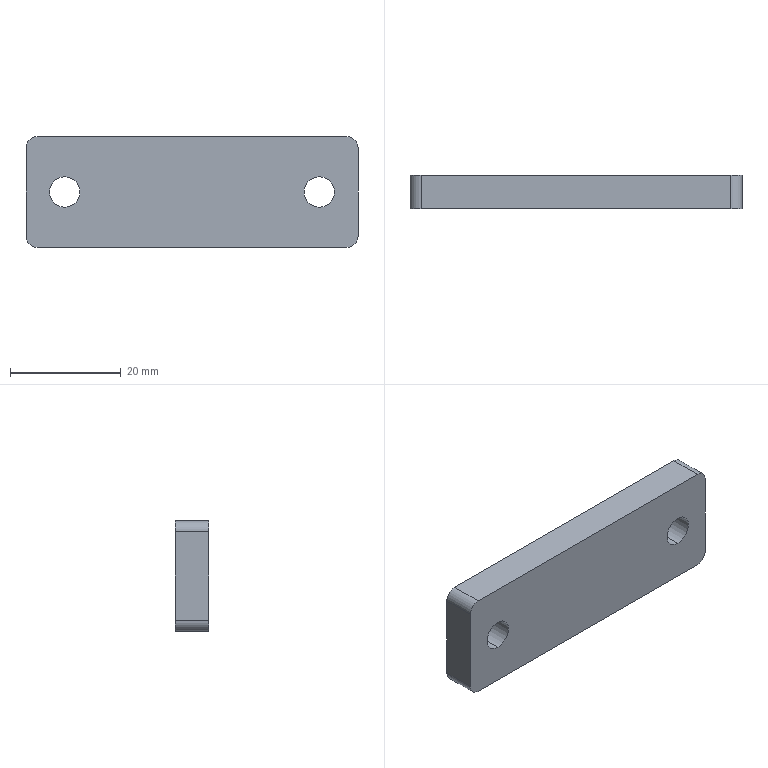Part | SolidWorks | features BaseBody 1 | 1 solid | 14 faces | box 60 x 6 x 20 mm | volume 6894 mm3 | cylinder 8 | plane 6 | commonest cylinder face diameters 4 x4 5.5 x4
STEP:
#1=CARTESIAN_POINT('',(23.,6.,2.75));
#2=VERTEX_POINT('',#1);
#3=CARTESIAN_POINT('',(23.,6.,-2.75));
#4=VERTEX_POINT('',#3);
#5=CARTESIAN_POINT('',(23.,6.,0.));
#6=DIRECTION('',(0.,-1.,0.));
#7=DIRECTION('',(0.,0.,-1.));
#8=AXIS2_PLACEMENT_3D('',#5,#6,#7);
#9=CIRCLE('',#8,2.75);
#10=EDGE_CURVE('',#2,#4,#9,.T.);
#11=ORIENTED_EDGE('',*,*,#10,.F.);
#12=CARTESIAN_POINT('',(23.,0.,2.75));
#13=VERTEX_POINT('',#12);
#14=CARTESIAN_POINT('',(23.,6.,2.75));
#15=DIRECTION('',(0.,-1.,0.));
#16=VECTOR('',#15,1000.);
#17=LINE('',#14,#16);
#18=EDGE_CURVE('',#2,#13,#17,.T.);
#19=ORIENTED_EDGE('',*,*,#18,.T.);
#20=CARTESIAN_POINT('',(23.,0.,-2.75));
#21=VERTEX_POINT('',#20);
#22=CARTESIAN_POINT('',(23.,0.,0.));
#23=DIRECTION('',(0.,1.,0.));
#24=DIRECTION('',(0.,0.,-1.));
#25=AXIS2_PLACEMENT_3D('',#22,#23,#24);
#26=CIRCLE('',#25,2.75);
#27=EDGE_CURVE('',#21,#13,#26,.T.);
#28=ORIENTED_EDGE('',*,*,#27,.F.);
#29=CARTESIAN_POINT('',(23.,6.,-2.75));
#30=DIRECTION('',(0.,-1.,0.));
#31=VECTOR('',#30,1000.);
#32=LINE('',#29,#31);
#33=EDGE_CURVE('',#4,#21,#32,.T.);
#34=ORIENTED_EDGE('',*,*,#33,.F.);
#35=EDGE_LOOP('',(#11,#19,#28,#34));
#36=FACE_OUTER_BOUND('',#35,.T.);
#37=CARTESIAN_POINT('',(23.,6.,0.));
#38=DIRECTION('',(0.,-1.,0.));
#39=DIRECTION('',(0.,0.,-1.));
#40=AXIS2_PLACEMENT_3D('',#37,#38,#39);
#41=CYLINDRICAL_SURFACE('',#40,2.75);
#42=ADVANCED_FACE('',(#36),#41,.F.);
#43=CARTESIAN_POINT('',(-23.,6.,2.75));
#44=VERTEX_POINT('',#43);
#45=CARTESIAN_POINT('',(-23.,6.,-2.75));
#46=VERTEX_POINT('',#45);
#47=CARTESIAN_POINT('',(-23.,6.,0.));
#48=DIRECTION('',(0.,-1.,0.));
#49=DIRECTION('',(0.,0.,-1.));
#50=AXIS2_PLACEMENT_3D('',#47,#48,#49);
#51=CIRCLE('',#50,2.75);
#52=EDGE_CURVE('',#44,#46,#51,.T.);
#53=ORIENTED_EDGE('',*,*,#52,.F.);
#54=CARTESIAN_POINT('',(-23.,0.,2.75));
#55=VERTEX_POINT('',#54);
#56=CARTESIAN_POINT('',(-23.,6.,2.75));
#57=DIRECTION('',(0.,-1.,0.));
#58=VECTOR('',#57,1000.);
#59=LINE('',#56,#58);
#60=EDGE_CURVE('',#44,#55,#59,.T.);
#61=ORIENTED_EDGE('',*,*,#60,.T.);
#62=CARTESIAN_POINT('',(-23.,0.,-2.75));
#63=VERTEX_POINT('',#62);
#64=CARTESIAN_POINT('',(-23.,0.,0.));
#65=DIRECTION('',(0.,1.,0.));
#66=DIRECTION('',(0.,0.,-1.));
#67=AXIS2_PLACEMENT_3D('',#64,#65,#66);
#68=CIRCLE('',#67,2.75);
#69=EDGE_CURVE('',#63,#55,#68,.T.);
#70=ORIENTED_EDGE('',*,*,#69,.F.);
#71=CARTESIAN_POINT('',(-23.,6.,-2.75));
#72=DIRECTION('',(0.,-1.,0.));
#73=VECTOR('',#72,1000.);
#74=LINE('',#71,#73);
#75=EDGE_CURVE('',#46,#63,#74,.T.);
#76=ORIENTED_EDGE('',*,*,#75,.F.);
#77=EDGE_LOOP('',(#53,#61,#70,#76));
#78=FACE_OUTER_BOUND('',#77,.T.);
#79=CARTESIAN_POINT('',(-23.,6.,0.));
#80=DIRECTION('',(0.,-1.,0.));
#81=DIRECTION('',(0.,0.,-1.));
#82=AXIS2_PLACEMENT_3D('',#79,#80,#81);
#83=CYLINDRICAL_SURFACE('',#82,2.75);
#84=ADVANCED_FACE('',(#78),#83,.F.);
#85=CARTESIAN_POINT('',(23.,6.,0.));
#86=DIRECTION('',(0.,-1.,0.));
#87=DIRECTION('',(0.,0.,-1.));
#88=AXIS2_PLACEMENT_3D('',#85,#86,#87);
#89=CIRCLE('',#88,2.75);
#90=EDGE_CURVE('',#4,#2,#89,.T.);
#91=ORIENTED_EDGE('',*,*,#90,.T.);
#92=ORIENTED_EDGE('',*,*,#10,.T.);
#93=EDGE_LOOP('',(#91,#92));
#94=FACE_BOUND('',#93,.T.);
#95=CARTESIAN_POINT('',(-30.,6.,-8.));
#96=VERTEX_POINT('',#95);
#97=CARTESIAN_POINT('',(-30.,6.,8.));
#98=VERTEX_POINT('',#97);
#99=CARTESIAN_POINT('',(-30.,6.,0.));
#100=DIRECTION('',(0.,0.,1.));
#101=VECTOR('',#100,1000.);
#102=LINE('',#99,#101);
#103=EDGE_CURVE('',#96,#98,#102,.T.);
#104=ORIENTED_EDGE('',*,*,#103,.T.);
#105=CARTESIAN_POINT('',(-28.,6.,10.));
#106=VERTEX_POINT('',#105);
#107=CARTESIAN_POINT('',(-28.,6.,8.));
#108=DIRECTION('',(0.,1.,0.));
#109=DIRECTION('',(0.,0.,-1.));
#110=AXIS2_PLACEMENT_3D('',#107,#108,#109);
#111=CIRCLE('',#110,2.);
#112=EDGE_CURVE('',#98,#106,#111,.T.);
#113=ORIENTED_EDGE('',*,*,#112,.T.);
#114=CARTESIAN_POINT('',(28.,6.,10.));
#115=VERTEX_POINT('',#114);
#116=CARTESIAN_POINT('',(0.,6.,10.));
#117=DIRECTION('',(1.,0.,0.));
#118=VECTOR('',#117,1000.);
#119=LINE('',#116,#118);
#120=EDGE_CURVE('',#106,#115,#119,.T.);
#121=ORIENTED_EDGE('',*,*,#120,.T.);
#122=CARTESIAN_POINT('',(30.,6.,8.));
#123=VERTEX_POINT('',#122);
#124=CARTESIAN_POINT('',(28.,6.,8.));
#125=DIRECTION('',(0.,1.,0.));
#126=DIRECTION('',(0.,0.,-1.));
#127=AXIS2_PLACEMENT_3D('',#124,#125,#126);
#128=CIRCLE('',#127,2.);
#129=EDGE_CURVE('',#115,#123,#128,.T.);
#130=ORIENTED_EDGE('',*,*,#129,.T.);
#131=CARTESIAN_POINT('',(30.,6.,-8.));
#132=VERTEX_POINT('',#131);
#133=CARTESIAN_POINT('',(30.,6.,0.));
#134=DIRECTION('',(0.,0.,-1.));
#135=VECTOR('',#134,1000.);
#136=LINE('',#133,#135);
#137=EDGE_CURVE('',#123,#132,#136,.T.);
#138=ORIENTED_EDGE('',*,*,#137,.T.);
#139=CARTESIAN_POINT('',(28.,6.,-10.));
#140=VERTEX_POINT('',#139);
#141=CARTESIAN_POINT('',(28.,6.,-8.));
#142=DIRECTION('',(0.,1.,0.));
#143=DIRECTION('',(0.,0.,-1.));
#144=AXIS2_PLACEMENT_3D('',#141,#142,#143);
#145=CIRCLE('',#144,2.);
#146=EDGE_CURVE('',#132,#140,#145,.T.);
#147=ORIENTED_EDGE('',*,*,#146,.T.);
#148=CARTESIAN_POINT('',(-28.,6.,-10.));
#149=VERTEX_POINT('',#148);
#150=CARTESIAN_POINT('',(0.,6.,-10.));
#151=DIRECTION('',(-1.,0.,0.));
#152=VECTOR('',#151,1000.);
#153=LINE('',#150,#152);
#154=EDGE_CURVE('',#140,#149,#153,.T.);
#155=ORIENTED_EDGE('',*,*,#154,.T.);
#156=CARTESIAN_POINT('',(-28.,6.,-8.));
#157=DIRECTION('',(0.,1.,0.));
#158=DIRECTION('',(0.,0.,-1.));
#159=AXIS2_PLACEMENT_3D('',#156,#157,#158);
#160=CIRCLE('',#159,2.);
#161=EDGE_CURVE('',#149,#96,#160,.T.);
#162=ORIENTED_EDGE('',*,*,#161,.T.);
#163=EDGE_LOOP('',(#104,#113,#121,#130,#138,#147,#155,#162));
#164=FACE_OUTER_BOUND('',#163,.T.);
#165=CARTESIAN_POINT('',(-23.,6.,0.));
#166=DIRECTION('',(0.,-1.,0.));
#167=DIRECTION('',(0.,0.,-1.));
#168=AXIS2_PLACEMENT_3D('',#165,#166,#167);
#169=CIRCLE('',#168,2.75);
#170=EDGE_CURVE('',#46,#44,#169,.T.);
#171=ORIENTED_EDGE('',*,*,#170,.T.);
#172=ORIENTED_EDGE('',*,*,#52,.T.);
#173=EDGE_LOOP('',(#171,#172));
#174=FACE_BOUND('',#173,.T.);
#175=CARTESIAN_POINT('',(0.,6.,0.));
#176=DIRECTION('',(0.,1.,0.));
#177=DIRECTION('',(0.,0.,1.));
#178=AXIS2_PLACEMENT_3D('',#175,#176,#177);
#179=PLANE('',#178);
#180=ADVANCED_FACE('',(#94,#164,#174),#179,.T.);
#181=ORIENTED_EDGE('',*,*,#18,.F.);
#182=ORIENTED_EDGE('',*,*,#90,.F.);
#183=ORIENTED_EDGE('',*,*,#33,.T.);
#184=CARTESIAN_POINT('',(23.,0.,0.));
#185=DIRECTION('',(0.,1.,0.));
#186=DIRECTION('',(0.,0.,-1.));
#187=AXIS2_PLACEMENT_3D('',#184,#185,#186);
#188=CIRCLE('',#187,2.75);
#189=EDGE_CURVE('',#13,#21,#188,.T.);
#190=ORIENTED_EDGE('',*,*,#189,.F.);
#191=EDGE_LOOP('',(#181,#182,#183,#190));
#192=FACE_OUTER_BOUND('',#191,.T.);
#193=CARTESIAN_POINT('',(23.,6.,0.));
#194=DIRECTION('',(0.,-1.,0.));
#195=DIRECTION('',(0.,0.,-1.));
#196=AXIS2_PLACEMENT_3D('',#193,#194,#195);
#197=CYLINDRICAL_SURFACE('',#196,2.75);
#198=ADVANCED_FACE('',(#192),#197,.F.);
#199=CARTESIAN_POINT('',(-30.,0.,8.));
#200=VERTEX_POINT('',#199);
#201=CARTESIAN_POINT('',(-28.,0.,10.));
#202=VERTEX_POINT('',#201);
#203=CARTESIAN_POINT('',(-28.,0.,8.));
#204=DIRECTION('',(0.,1.,0.));
#205=DIRECTION('',(0.,0.,-1.));
#206=AXIS2_PLACEMENT_3D('',#203,#204,#205);
#207=CIRCLE('',#206,2.);
#208=EDGE_CURVE('',#200,#202,#207,.T.);
#209=ORIENTED_EDGE('',*,*,#208,.T.);
#210=CARTESIAN_POINT('',(-28.,6.,10.));
#211=DIRECTION('',(0.,1.,0.));
#212=VECTOR('',#211,1000.);
#213=LINE('',#210,#212);
#214=EDGE_CURVE('',#202,#106,#213,.T.);
#215=ORIENTED_EDGE('',*,*,#214,.T.);
#216=ORIENTED_EDGE('',*,*,#112,.F.);
#217=CARTESIAN_POINT('',(-30.,6.,8.));
#218=DIRECTION('',(0.,-1.,0.));
#219=VECTOR('',#218,1000.);
#220=LINE('',#217,#219);
#221=EDGE_CURVE('',#98,#200,#220,.T.);
#222=ORIENTED_EDGE('',*,*,#221,.T.);
#223=EDGE_LOOP('',(#209,#215,#216,#222));
#224=FACE_OUTER_BOUND('',#223,.T.);
#225=CARTESIAN_POINT('',(-28.,6.,8.));
#226=DIRECTION('',(0.,-1.,0.));
#227=DIRECTION('',(0.,0.,-1.));
#228=AXIS2_PLACEMENT_3D('',#225,#226,#227);
#229=CYLINDRICAL_SURFACE('',#228,2.);
#230=ADVANCED_FACE('',(#224),#229,.T.);
#231=ORIENTED_EDGE('',*,*,#221,.F.);
#232=ORIENTED_EDGE('',*,*,#103,.F.);
#233=CARTESIAN_POINT('',(-30.,0.,-8.));
#234=VERTEX_POINT('',#233);
#235=CARTESIAN_POINT('',(-30.,6.,-8.));
#236=DIRECTION('',(0.,1.,0.));
#237=VECTOR('',#236,1000.);
#238=LINE('',#235,#237);
#239=EDGE_CURVE('',#234,#96,#238,.T.);
#240=ORIENTED_EDGE('',*,*,#239,.F.);
#241=CARTESIAN_POINT('',(-30.,0.,10.));
#242=DIRECTION('',(0.,0.,-1.));
#243=VECTOR('',#242,1000.);
#244=LINE('',#241,#243);
#245=EDGE_CURVE('',#200,#234,#244,.T.);
#246=ORIENTED_EDGE('',*,*,#245,.F.);
#247=EDGE_LOOP('',(#231,#232,#240,#246));
#248=FACE_OUTER_BOUND('',#247,.T.);
#249=CARTESIAN_POINT('',(-30.,6.,10.));
#250=DIRECTION('',(1.,0.,0.));
#251=DIRECTION('',(0.,0.,-1.));
#252=AXIS2_PLACEMENT_3D('',#249,#250,#251);
#253=PLANE('',#252);
#254=ADVANCED_FACE('',(#248),#253,.F.);
#255=CARTESIAN_POINT('',(-28.,0.,-10.));
#256=VERTEX_POINT('',#255);
#257=CARTESIAN_POINT('',(-28.,0.,-8.));
#258=DIRECTION('',(0.,1.,0.));
#259=DIRECTION('',(0.,0.,-1.));
#260=AXIS2_PLACEMENT_3D('',#257,#258,#259);
#261=CIRCLE('',#260,2.);
#262=EDGE_CURVE('',#256,#234,#261,.T.);
#263=ORIENTED_EDGE('',*,*,#262,.T.);
#264=ORIENTED_EDGE('',*,*,#239,.T.);
#265=ORIENTED_EDGE('',*,*,#161,.F.);
#266=CARTESIAN_POINT('',(-28.,6.,-10.));
#267=DIRECTION('',(0.,-1.,0.));
#268=VECTOR('',#267,1000.);
#269=LINE('',#266,#268);
#270=EDGE_CURVE('',#149,#256,#269,.T.);
#271=ORIENTED_EDGE('',*,*,#270,.T.);
#272=EDGE_LOOP('',(#263,#264,#265,#271));
#273=FACE_OUTER_BOUND('',#272,.T.);
#274=CARTESIAN_POINT('',(-28.,6.,-8.));
#275=DIRECTION('',(0.,-1.,0.));
#276=DIRECTION('',(0.,0.,-1.));
#277=AXIS2_PLACEMENT_3D('',#274,#275,#276);
#278=CYLINDRICAL_SURFACE('',#277,2.);
#279=ADVANCED_FACE('',(#273),#278,.T.);
#280=CARTESIAN_POINT('',(28.,0.,-10.));
#281=VERTEX_POINT('',#280);
#282=CARTESIAN_POINT('',(28.,6.,-10.));
#283=DIRECTION('',(0.,1.,0.));
#284=VECTOR('',#283,1000.);
#285=LINE('',#282,#284);
#286=EDGE_CURVE('',#281,#140,#285,.T.);
#287=ORIENTED_EDGE('',*,*,#286,.F.);
#288=CARTESIAN_POINT('',(30.,0.,-10.));
#289=DIRECTION('',(1.,0.,0.));
#290=VECTOR('',#289,1000.);
#291=LINE('',#288,#290);
#292=EDGE_CURVE('',#256,#281,#291,.T.);
#293=ORIENTED_EDGE('',*,*,#292,.F.);
#294=ORIENTED_EDGE('',*,*,#270,.F.);
#295=ORIENTED_EDGE('',*,*,#154,.F.);
#296=EDGE_LOOP('',(#287,#293,#294,#295));
#297=FACE_OUTER_BOUND('',#296,.T.);
#298=CARTESIAN_POINT('',(30.,6.,-10.));
#299=DIRECTION('',(0.,0.,1.));
#300=DIRECTION('',(1.,0.,0.));
#301=AXIS2_PLACEMENT_3D('',#298,#299,#300);
#302=PLANE('',#301);
#303=ADVANCED_FACE('',(#297),#302,.F.);
#304=CARTESIAN_POINT('',(30.,0.,-8.));
#305=VERTEX_POINT('',#304);
#306=CARTESIAN_POINT('',(28.,0.,-8.));
#307=DIRECTION('',(0.,1.,0.));
#308=DIRECTION('',(0.,0.,-1.));
#309=AXIS2_PLACEMENT_3D('',#306,#307,#308);
#310=CIRCLE('',#309,2.);
#311=EDGE_CURVE('',#305,#281,#310,.T.);
#312=ORIENTED_EDGE('',*,*,#311,.T.);
#313=ORIENTED_EDGE('',*,*,#286,.T.);
#314=ORIENTED_EDGE('',*,*,#146,.F.);
#315=CARTESIAN_POINT('',(30.,6.,-8.));
#316=DIRECTION('',(0.,-1.,0.));
#317=VECTOR('',#316,1000.);
#318=LINE('',#315,#317);
#319=EDGE_CURVE('',#132,#305,#318,.T.);
#320=ORIENTED_EDGE('',*,*,#319,.T.);
#321=EDGE_LOOP('',(#312,#313,#314,#320));
#322=FACE_OUTER_BOUND('',#321,.T.);
#323=CARTESIAN_POINT('',(28.,6.,-8.));
#324=DIRECTION('',(0.,-1.,0.));
#325=DIRECTION('',(0.,0.,-1.));
#326=AXIS2_PLACEMENT_3D('',#323,#324,#325);
#327=CYLINDRICAL_SURFACE('',#326,2.);
#328=ADVANCED_FACE('',(#322),#327,.T.);
#329=CARTESIAN_POINT('',(30.,0.,8.));
#330=VERTEX_POINT('',#329);
#331=CARTESIAN_POINT('',(30.,6.,8.));
#332=DIRECTION('',(0.,1.,0.));
#333=VECTOR('',#332,1000.);
#334=LINE('',#331,#333);
#335=EDGE_CURVE('',#330,#123,#334,.T.);
#336=ORIENTED_EDGE('',*,*,#335,.F.);
#337=CARTESIAN_POINT('',(30.,0.,10.));
#338=DIRECTION('',(0.,0.,1.));
#339=VECTOR('',#338,1000.);
#340=LINE('',#337,#339);
#341=EDGE_CURVE('',#305,#330,#340,.T.);
#342=ORIENTED_EDGE('',*,*,#341,.F.);
#343=ORIENTED_EDGE('',*,*,#319,.F.);
#344=ORIENTED_EDGE('',*,*,#137,.F.);
#345=EDGE_LOOP('',(#336,#342,#343,#344));
#346=FACE_OUTER_BOUND('',#345,.T.);
#347=CARTESIAN_POINT('',(30.,6.,10.));
#348=DIRECTION('',(-1.,0.,0.));
#349=DIRECTION('',(0.,0.,1.));
#350=AXIS2_PLACEMENT_3D('',#347,#348,#349);
#351=PLANE('',#350);
#352=ADVANCED_FACE('',(#346),#351,.F.);
#353=CARTESIAN_POINT('',(28.,0.,10.));
#354=VERTEX_POINT('',#353);
#355=CARTESIAN_POINT('',(28.,0.,8.));
#356=DIRECTION('',(0.,1.,0.));
#357=DIRECTION('',(0.,0.,-1.));
#358=AXIS2_PLACEMENT_3D('',#355,#356,#357);
#359=CIRCLE('',#358,2.);
#360=EDGE_CURVE('',#354,#330,#359,.T.);
#361=ORIENTED_EDGE('',*,*,#360,.T.);
#362=ORIENTED_EDGE('',*,*,#335,.T.);
#363=ORIENTED_EDGE('',*,*,#129,.F.);
#364=CARTESIAN_POINT('',(28.,6.,10.));
#365=DIRECTION('',(0.,-1.,0.));
#366=VECTOR('',#365,1000.);
#367=LINE('',#364,#366);
#368=EDGE_CURVE('',#115,#354,#367,.T.);
#369=ORIENTED_EDGE('',*,*,#368,.T.);
#370=EDGE_LOOP('',(#361,#362,#363,#369));
#371=FACE_OUTER_BOUND('',#370,.T.);
#372=CARTESIAN_POINT('',(28.,6.,8.));
#373=DIRECTION('',(0.,-1.,0.));
#374=DIRECTION('',(0.,0.,-1.));
#375=AXIS2_PLACEMENT_3D('',#372,#373,#374);
#376=CYLINDRICAL_SURFACE('',#375,2.);
#377=ADVANCED_FACE('',(#371),#376,.T.);
#378=ORIENTED_EDGE('',*,*,#368,.F.);
#379=ORIENTED_EDGE('',*,*,#120,.F.);
#380=ORIENTED_EDGE('',*,*,#214,.F.);
#381=CARTESIAN_POINT('',(30.,0.,10.));
#382=DIRECTION('',(-1.,0.,0.));
#383=VECTOR('',#382,1000.);
#384=LINE('',#381,#383);
#385=EDGE_CURVE('',#354,#202,#384,.T.);
#386=ORIENTED_EDGE('',*,*,#385,.F.);
#387=EDGE_LOOP('',(#378,#379,#380,#386));
#388=FACE_OUTER_BOUND('',#387,.T.);
#389=CARTESIAN_POINT('',(30.,6.,10.));
#390=DIRECTION('',(0.,0.,-1.));
#391=DIRECTION('',(-1.,0.,0.));
#392=AXIS2_PLACEMENT_3D('',#389,#390,#391);
#393=PLANE('',#392);
#394=ADVANCED_FACE('',(#388),#393,.F.);
#395=ORIENTED_EDGE('',*,*,#60,.F.);
#396=ORIENTED_EDGE('',*,*,#170,.F.);
#397=ORIENTED_EDGE('',*,*,#75,.T.);
#398=CARTESIAN_POINT('',(-23.,0.,0.));
#399=DIRECTION('',(0.,1.,0.));
#400=DIRECTION('',(0.,0.,-1.));
#401=AXIS2_PLACEMENT_3D('',#398,#399,#400);
#402=CIRCLE('',#401,2.75);
#403=EDGE_CURVE('',#55,#63,#402,.T.);
#404=ORIENTED_EDGE('',*,*,#403,.F.);
#405=EDGE_LOOP('',(#395,#396,#397,#404));
#406=FACE_OUTER_BOUND('',#405,.T.);
#407=CARTESIAN_POINT('',(-23.,6.,0.));
#408=DIRECTION('',(0.,-1.,0.));
#409=DIRECTION('',(0.,0.,-1.));
#410=AXIS2_PLACEMENT_3D('',#407,#408,#409);
#411=CYLINDRICAL_SURFACE('',#410,2.75);
#412=ADVANCED_FACE('',(#406),#411,.F.);
#413=ORIENTED_EDGE('',*,*,#27,.T.);
#414=ORIENTED_EDGE('',*,*,#189,.T.);
#415=EDGE_LOOP('',(#413,#414));
#416=FACE_BOUND('',#415,.T.);
#417=ORIENTED_EDGE('',*,*,#69,.T.);
#418=ORIENTED_EDGE('',*,*,#403,.T.);
#419=EDGE_LOOP('',(#417,#418));
#420=FACE_BOUND('',#419,.T.);
#421=ORIENTED_EDGE('',*,*,#360,.F.);
#422=ORIENTED_EDGE('',*,*,#385,.T.);
#423=ORIENTED_EDGE('',*,*,#208,.F.);
#424=ORIENTED_EDGE('',*,*,#245,.T.);
#425=ORIENTED_EDGE('',*,*,#262,.F.);
#426=ORIENTED_EDGE('',*,*,#292,.T.);
#427=ORIENTED_EDGE('',*,*,#311,.F.);
#428=ORIENTED_EDGE('',*,*,#341,.T.);
#429=EDGE_LOOP('',(#421,#422,#423,#424,#425,#426,#427,#428));
#430=FACE_OUTER_BOUND('',#429,.T.);
#431=CARTESIAN_POINT('',(0.,0.,0.));
#432=DIRECTION('',(0.,1.,0.));
#433=DIRECTION('',(0.,0.,1.));
#434=AXIS2_PLACEMENT_3D('',#431,#432,#433);
#435=PLANE('',#434);
#436=ADVANCED_FACE('',(#416,#420,#430),#435,.F.);
#437=CLOSED_SHELL('',(#42,#84,#180,#198,#230,#254,#279,#303,#328,#352,#377,#394,#412,#436));
#438=MANIFOLD_SOLID_BREP('',#437);
#439=CARTESIAN_POINT('',(0.,0.,0.));
#440=DIRECTION('',(0.,0.,1.));
#441=DIRECTION('',(1.,0.,0.));
#442=AXIS2_PLACEMENT_3D('',#439,#440,#441);
#443=(LENGTH_UNIT()NAMED_UNIT(*)SI_UNIT(.MILLI.,.METRE.));
#444=UNCERTAINTY_MEASURE_WITH_UNIT(LENGTH_MEASURE(0.00001),#443,'','');
#445=(NAMED_UNIT(*)PLANE_ANGLE_UNIT()SI_UNIT($,.RADIAN.));
#446=(NAMED_UNIT(*)SI_UNIT($,.STERADIAN.)SOLID_ANGLE_UNIT());
#447=(GEOMETRIC_REPRESENTATION_CONTEXT(3)GLOBAL_UNCERTAINTY_ASSIGNED_CONTEXT((#444))GLOBAL_UNIT_ASSIGNED_CONTEXT((#443,#445,#446))REPRESENTATION_CONTEXT('',''));
#448=ADVANCED_BREP_SHAPE_REPRESENTATION('',(#438,#442),#447);